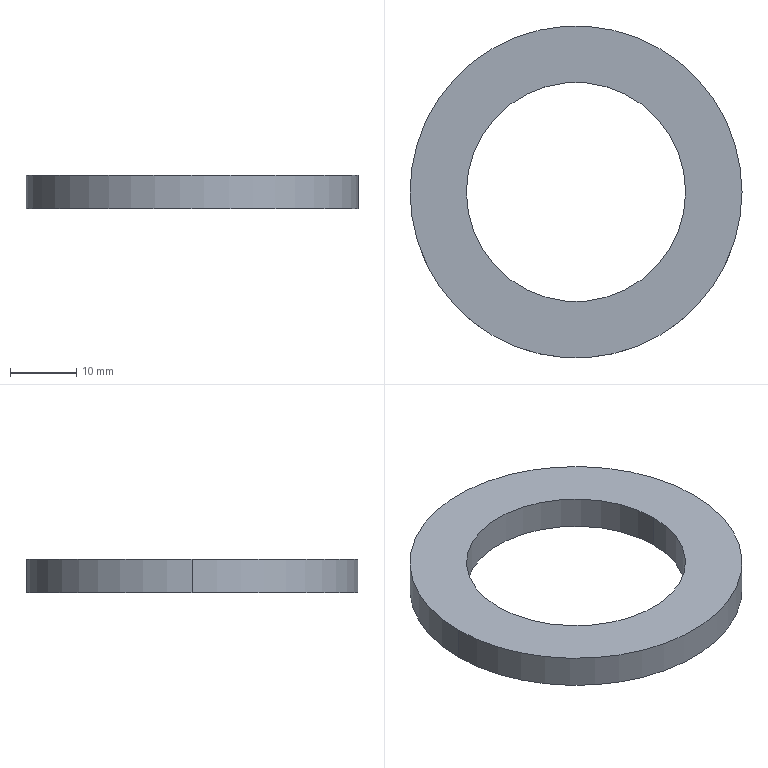Part | SolidWorks | features BaseBody 1 | 1 solid | 6 faces | box 50 x 50 x 5 mm | volume 5541 mm3 | cylinder 4 | plane 2 | commonest cylinder face diameters 33 x2 50 x2
STEP:
#1=CARTESIAN_POINT('',(-47.479,21.276,5.));
#2=VERTEX_POINT('',#1);
#3=CARTESIAN_POINT('',(-80.479,21.276,5.));
#4=VERTEX_POINT('',#3);
#5=CARTESIAN_POINT('',(-63.979,21.276,5.));
#6=DIRECTION('',(0.,0.,-1.));
#7=DIRECTION('',(-1.,0.,0.));
#8=AXIS2_PLACEMENT_3D('',#5,#6,#7);
#9=CIRCLE('',#8,16.5);
#10=EDGE_CURVE('',#2,#4,#9,.T.);
#11=ORIENTED_EDGE('',*,*,#10,.F.);
#12=CARTESIAN_POINT('',(-47.479,21.276,0.));
#13=VERTEX_POINT('',#12);
#14=CARTESIAN_POINT('',(-47.479,21.276,5.));
#15=DIRECTION('',(0.,0.,-1.));
#16=VECTOR('',#15,1000.);
#17=LINE('',#14,#16);
#18=EDGE_CURVE('',#2,#13,#17,.T.);
#19=ORIENTED_EDGE('',*,*,#18,.T.);
#20=CARTESIAN_POINT('',(-80.479,21.276,0.));
#21=VERTEX_POINT('',#20);
#22=CARTESIAN_POINT('',(-63.979,21.276,0.));
#23=DIRECTION('',(0.,0.,1.));
#24=DIRECTION('',(-1.,0.,0.));
#25=AXIS2_PLACEMENT_3D('',#22,#23,#24);
#26=CIRCLE('',#25,16.5);
#27=EDGE_CURVE('',#21,#13,#26,.T.);
#28=ORIENTED_EDGE('',*,*,#27,.F.);
#29=CARTESIAN_POINT('',(-80.479,21.276,5.));
#30=DIRECTION('',(0.,0.,-1.));
#31=VECTOR('',#30,1000.);
#32=LINE('',#29,#31);
#33=EDGE_CURVE('',#4,#21,#32,.T.);
#34=ORIENTED_EDGE('',*,*,#33,.F.);
#35=EDGE_LOOP('',(#11,#19,#28,#34));
#36=FACE_OUTER_BOUND('',#35,.T.);
#37=CARTESIAN_POINT('',(-63.979,21.276,5.));
#38=DIRECTION('',(0.,0.,-1.));
#39=DIRECTION('',(-1.,0.,0.));
#40=AXIS2_PLACEMENT_3D('',#37,#38,#39);
#41=CYLINDRICAL_SURFACE('',#40,16.5);
#42=ADVANCED_FACE('',(#36),#41,.F.);
#43=CARTESIAN_POINT('',(-38.979,21.276,5.));
#44=VERTEX_POINT('',#43);
#45=CARTESIAN_POINT('',(-88.979,21.276,5.));
#46=VERTEX_POINT('',#45);
#47=CARTESIAN_POINT('',(-63.979,21.276,5.));
#48=DIRECTION('',(0.,0.,1.));
#49=DIRECTION('',(-1.,0.,0.));
#50=AXIS2_PLACEMENT_3D('',#47,#48,#49);
#51=CIRCLE('',#50,25.);
#52=EDGE_CURVE('',#44,#46,#51,.T.);
#53=ORIENTED_EDGE('',*,*,#52,.F.);
#54=CARTESIAN_POINT('',(-38.979,21.276,0.));
#55=VERTEX_POINT('',#54);
#56=CARTESIAN_POINT('',(-38.979,21.276,5.));
#57=DIRECTION('',(0.,0.,-1.));
#58=VECTOR('',#57,1000.);
#59=LINE('',#56,#58);
#60=EDGE_CURVE('',#44,#55,#59,.T.);
#61=ORIENTED_EDGE('',*,*,#60,.T.);
#62=CARTESIAN_POINT('',(-88.979,21.276,0.));
#63=VERTEX_POINT('',#62);
#64=CARTESIAN_POINT('',(-63.979,21.276,0.));
#65=DIRECTION('',(0.,0.,1.));
#66=DIRECTION('',(-1.,0.,0.));
#67=AXIS2_PLACEMENT_3D('',#64,#65,#66);
#68=CIRCLE('',#67,25.);
#69=EDGE_CURVE('',#55,#63,#68,.T.);
#70=ORIENTED_EDGE('',*,*,#69,.T.);
#71=CARTESIAN_POINT('',(-88.979,21.276,5.));
#72=DIRECTION('',(0.,0.,-1.));
#73=VECTOR('',#72,1000.);
#74=LINE('',#71,#73);
#75=EDGE_CURVE('',#46,#63,#74,.T.);
#76=ORIENTED_EDGE('',*,*,#75,.F.);
#77=EDGE_LOOP('',(#53,#61,#70,#76));
#78=FACE_OUTER_BOUND('',#77,.T.);
#79=CARTESIAN_POINT('',(-63.979,21.276,5.));
#80=DIRECTION('',(0.,0.,-1.));
#81=DIRECTION('',(-1.,0.,0.));
#82=AXIS2_PLACEMENT_3D('',#79,#80,#81);
#83=CYLINDRICAL_SURFACE('',#82,25.);
#84=ADVANCED_FACE('',(#78),#83,.T.);
#85=CARTESIAN_POINT('',(-63.979,21.276,5.));
#86=DIRECTION('',(0.,0.,-1.));
#87=DIRECTION('',(-1.,0.,0.));
#88=AXIS2_PLACEMENT_3D('',#85,#86,#87);
#89=CIRCLE('',#88,16.5);
#90=EDGE_CURVE('',#4,#2,#89,.T.);
#91=ORIENTED_EDGE('',*,*,#90,.T.);
#92=ORIENTED_EDGE('',*,*,#10,.T.);
#93=EDGE_LOOP('',(#91,#92));
#94=FACE_BOUND('',#93,.T.);
#95=CARTESIAN_POINT('',(-63.979,21.276,5.));
#96=DIRECTION('',(0.,0.,1.));
#97=DIRECTION('',(-1.,0.,0.));
#98=AXIS2_PLACEMENT_3D('',#95,#96,#97);
#99=CIRCLE('',#98,25.);
#100=EDGE_CURVE('',#46,#44,#99,.T.);
#101=ORIENTED_EDGE('',*,*,#100,.T.);
#102=ORIENTED_EDGE('',*,*,#52,.T.);
#103=EDGE_LOOP('',(#101,#102));
#104=FACE_OUTER_BOUND('',#103,.T.);
#105=CARTESIAN_POINT('',(-63.979,21.276,5.));
#106=DIRECTION('',(0.,0.,1.));
#107=DIRECTION('',(1.,0.,0.));
#108=AXIS2_PLACEMENT_3D('',#105,#106,#107);
#109=PLANE('',#108);
#110=ADVANCED_FACE('',(#94,#104),#109,.T.);
#111=ORIENTED_EDGE('',*,*,#18,.F.);
#112=ORIENTED_EDGE('',*,*,#90,.F.);
#113=ORIENTED_EDGE('',*,*,#33,.T.);
#114=CARTESIAN_POINT('',(-63.979,21.276,0.));
#115=DIRECTION('',(0.,0.,1.));
#116=DIRECTION('',(-1.,0.,0.));
#117=AXIS2_PLACEMENT_3D('',#114,#115,#116);
#118=CIRCLE('',#117,16.5);
#119=EDGE_CURVE('',#13,#21,#118,.T.);
#120=ORIENTED_EDGE('',*,*,#119,.F.);
#121=EDGE_LOOP('',(#111,#112,#113,#120));
#122=FACE_OUTER_BOUND('',#121,.T.);
#123=CARTESIAN_POINT('',(-63.979,21.276,5.));
#124=DIRECTION('',(0.,0.,-1.));
#125=DIRECTION('',(-1.,0.,0.));
#126=AXIS2_PLACEMENT_3D('',#123,#124,#125);
#127=CYLINDRICAL_SURFACE('',#126,16.5);
#128=ADVANCED_FACE('',(#122),#127,.F.);
#129=ORIENTED_EDGE('',*,*,#60,.F.);
#130=ORIENTED_EDGE('',*,*,#100,.F.);
#131=ORIENTED_EDGE('',*,*,#75,.T.);
#132=CARTESIAN_POINT('',(-63.979,21.276,0.));
#133=DIRECTION('',(0.,0.,1.));
#134=DIRECTION('',(-1.,0.,0.));
#135=AXIS2_PLACEMENT_3D('',#132,#133,#134);
#136=CIRCLE('',#135,25.);
#137=EDGE_CURVE('',#63,#55,#136,.T.);
#138=ORIENTED_EDGE('',*,*,#137,.T.);
#139=EDGE_LOOP('',(#129,#130,#131,#138));
#140=FACE_OUTER_BOUND('',#139,.T.);
#141=CARTESIAN_POINT('',(-63.979,21.276,5.));
#142=DIRECTION('',(0.,0.,-1.));
#143=DIRECTION('',(-1.,0.,0.));
#144=AXIS2_PLACEMENT_3D('',#141,#142,#143);
#145=CYLINDRICAL_SURFACE('',#144,25.);
#146=ADVANCED_FACE('',(#140),#145,.T.);
#147=ORIENTED_EDGE('',*,*,#27,.T.);
#148=ORIENTED_EDGE('',*,*,#119,.T.);
#149=EDGE_LOOP('',(#147,#148));
#150=FACE_BOUND('',#149,.T.);
#151=ORIENTED_EDGE('',*,*,#137,.F.);
#152=ORIENTED_EDGE('',*,*,#69,.F.);
#153=EDGE_LOOP('',(#151,#152));
#154=FACE_OUTER_BOUND('',#153,.T.);
#155=CARTESIAN_POINT('',(-63.979,21.276,0.));
#156=DIRECTION('',(0.,0.,1.));
#157=DIRECTION('',(1.,0.,0.));
#158=AXIS2_PLACEMENT_3D('',#155,#156,#157);
#159=PLANE('',#158);
#160=ADVANCED_FACE('',(#150,#154),#159,.F.);
#161=CLOSED_SHELL('',(#42,#84,#110,#128,#146,#160));
#162=MANIFOLD_SOLID_BREP('',#161);
#163=CARTESIAN_POINT('',(0.,0.,0.));
#164=DIRECTION('',(0.,0.,1.));
#165=DIRECTION('',(1.,0.,0.));
#166=AXIS2_PLACEMENT_3D('',#163,#164,#165);
#167=(LENGTH_UNIT()NAMED_UNIT(*)SI_UNIT(.MILLI.,.METRE.));
#168=UNCERTAINTY_MEASURE_WITH_UNIT(LENGTH_MEASURE(0.00001),#167,'','');
#169=(NAMED_UNIT(*)PLANE_ANGLE_UNIT()SI_UNIT($,.RADIAN.));
#170=(NAMED_UNIT(*)SI_UNIT($,.STERADIAN.)SOLID_ANGLE_UNIT());
#171=(GEOMETRIC_REPRESENTATION_CONTEXT(3)GLOBAL_UNCERTAINTY_ASSIGNED_CONTEXT((#168))GLOBAL_UNIT_ASSIGNED_CONTEXT((#167,#169,#170))REPRESENTATION_CONTEXT('',''));
#172=ADVANCED_BREP_SHAPE_REPRESENTATION('',(#162,#166),#171);